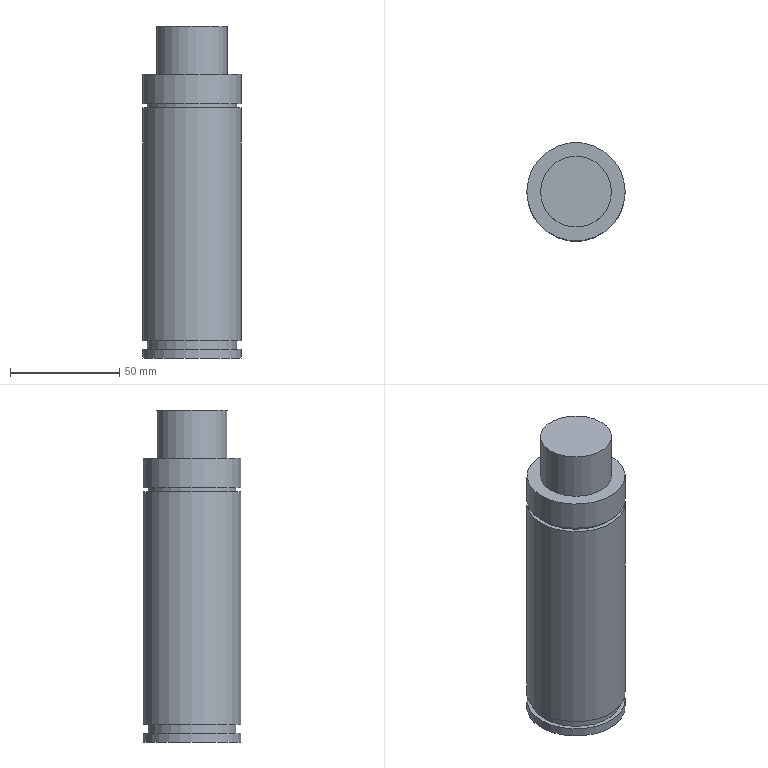Part | NX | features solid 2 | 1 solid | 13 faces | box 45 x 45 x 152 mm | volume 223386 mm3 | plane 7 | cylinder 6 | commonest cylinder face diameters 45 x3 41 x2 32.5 x1
STEP:
#1=CARTESIAN_POINT('',(-897.5,-460.,-46.99));
#2=VERTEX_POINT('',#1);
#3=CARTESIAN_POINT('',(-875.,-460.,-46.99));
#4=DIRECTION('',(0.,0.,1.));
#5=DIRECTION('',(-1.,0.,0.));
#6=AXIS2_PLACEMENT_3D('',#3,#4,#5);
#7=CIRCLE('',#6,22.5);
#8=EDGE_CURVE('',#2,#2,#7,.T.);
#9=ORIENTED_EDGE('',*,*,#8,.T.);
#10=EDGE_LOOP('',(#9));
#11=FACE_BOUND('',#10,.T.);
#12=CARTESIAN_POINT('',(-897.5,-460.,59.51));
#13=VERTEX_POINT('',#12);
#14=CARTESIAN_POINT('',(-875.,-460.,59.51));
#15=DIRECTION('',(0.,0.,1.));
#16=DIRECTION('',(-1.,0.,0.));
#17=AXIS2_PLACEMENT_3D('',#14,#15,#16);
#18=CIRCLE('',#17,22.5);
#19=EDGE_CURVE('',#13,#13,#18,.T.);
#20=ORIENTED_EDGE('',*,*,#19,.F.);
#21=EDGE_LOOP('',(#20));
#22=FACE_BOUND('',#21,.T.);
#23=CARTESIAN_POINT('',(-875.,-460.,-54.99));
#24=DIRECTION('',(0.,0.,1.));
#25=DIRECTION('',(-1.,0.,0.));
#26=AXIS2_PLACEMENT_3D('',#23,#24,#25);
#27=CYLINDRICAL_SURFACE('',#26,22.5);
#28=ADVANCED_FACE('',(#11,#22),#27,.T.);
#29=CARTESIAN_POINT('',(-895.5,-460.,-46.99));
#30=VERTEX_POINT('',#29);
#31=CARTESIAN_POINT('',(-875.,-460.,-46.99));
#32=DIRECTION('',(0.,0.,1.));
#33=DIRECTION('',(-1.,0.,0.));
#34=AXIS2_PLACEMENT_3D('',#31,#32,#33);
#35=CIRCLE('',#34,20.5);
#36=EDGE_CURVE('',#30,#30,#35,.T.);
#37=ORIENTED_EDGE('',*,*,#36,.T.);
#38=EDGE_LOOP('',(#37));
#39=FACE_BOUND('',#38,.T.);
#40=ORIENTED_EDGE('',*,*,#8,.F.);
#41=EDGE_LOOP('',(#40));
#42=FACE_BOUND('',#41,.T.);
#43=CARTESIAN_POINT('',(-875.,-460.,-46.99));
#44=DIRECTION('',(0.,0.,-1.));
#45=DIRECTION('',(1.,0.,0.));
#46=AXIS2_PLACEMENT_3D('',#43,#44,#45);
#47=PLANE('',#46);
#48=ADVANCED_FACE('',(#39,#42),#47,.T.);
#49=CARTESIAN_POINT('',(-895.5,-460.,-50.99));
#50=VERTEX_POINT('',#49);
#51=CARTESIAN_POINT('',(-875.,-460.,-50.99));
#52=DIRECTION('',(0.,0.,1.));
#53=DIRECTION('',(-1.,0.,0.));
#54=AXIS2_PLACEMENT_3D('',#51,#52,#53);
#55=CIRCLE('',#54,20.5);
#56=EDGE_CURVE('',#50,#50,#55,.T.);
#57=ORIENTED_EDGE('',*,*,#56,.F.);
#58=EDGE_LOOP('',(#57));
#59=FACE_BOUND('',#58,.T.);
#60=CARTESIAN_POINT('',(-897.5,-460.,-50.99));
#61=VERTEX_POINT('',#60);
#62=CARTESIAN_POINT('',(-875.,-460.,-50.99));
#63=DIRECTION('',(0.,0.,1.));
#64=DIRECTION('',(-1.,0.,0.));
#65=AXIS2_PLACEMENT_3D('',#62,#63,#64);
#66=CIRCLE('',#65,22.5);
#67=EDGE_CURVE('',#61,#61,#66,.T.);
#68=ORIENTED_EDGE('',*,*,#67,.T.);
#69=EDGE_LOOP('',(#68));
#70=FACE_BOUND('',#69,.T.);
#71=CARTESIAN_POINT('',(-875.,-460.,-50.99));
#72=DIRECTION('',(0.,0.,-1.));
#73=DIRECTION('',(1.,0.,0.));
#74=AXIS2_PLACEMENT_3D('',#71,#72,#73);
#75=PLANE('',#74);
#76=ADVANCED_FACE('',(#59,#70),#75,.F.);
#77=ORIENTED_EDGE('',*,*,#36,.F.);
#78=EDGE_LOOP('',(#77));
#79=FACE_BOUND('',#78,.T.);
#80=ORIENTED_EDGE('',*,*,#56,.T.);
#81=EDGE_LOOP('',(#80));
#82=FACE_BOUND('',#81,.T.);
#83=CARTESIAN_POINT('',(-875.,-460.,-50.99));
#84=DIRECTION('',(0.,0.,1.));
#85=DIRECTION('',(-1.,0.,0.));
#86=AXIS2_PLACEMENT_3D('',#83,#84,#85);
#87=CYLINDRICAL_SURFACE('',#86,20.5);
#88=ADVANCED_FACE('',(#79,#82),#87,.T.);
#89=CARTESIAN_POINT('',(-897.5,-460.,-54.99));
#90=VERTEX_POINT('',#89);
#91=CARTESIAN_POINT('',(-875.,-460.,-54.99));
#92=DIRECTION('',(0.,0.,1.));
#93=DIRECTION('',(-1.,0.,0.));
#94=AXIS2_PLACEMENT_3D('',#91,#92,#93);
#95=CIRCLE('',#94,22.5);
#96=EDGE_CURVE('',#90,#90,#95,.T.);
#97=ORIENTED_EDGE('',*,*,#96,.F.);
#98=EDGE_LOOP('',(#97));
#99=FACE_BOUND('',#98,.T.);
#100=CARTESIAN_POINT('',(-875.,-460.,-54.99));
#101=DIRECTION('',(0.,0.,1.));
#102=DIRECTION('',(-1.,0.,0.));
#103=AXIS2_PLACEMENT_3D('',#100,#101,#102);
#104=PLANE('',#103);
#105=ADVANCED_FACE('',(#99),#104,.F.);
#106=ORIENTED_EDGE('',*,*,#96,.T.);
#107=EDGE_LOOP('',(#106));
#108=FACE_BOUND('',#107,.T.);
#109=ORIENTED_EDGE('',*,*,#67,.F.);
#110=EDGE_LOOP('',(#109));
#111=FACE_BOUND('',#110,.T.);
#112=CARTESIAN_POINT('',(-875.,-460.,-54.99));
#113=DIRECTION('',(0.,0.,1.));
#114=DIRECTION('',(-1.,0.,0.));
#115=AXIS2_PLACEMENT_3D('',#112,#113,#114);
#116=CYLINDRICAL_SURFACE('',#115,22.5);
#117=ADVANCED_FACE('',(#108,#111),#116,.T.);
#118=CARTESIAN_POINT('',(-854.5,-460.,59.51));
#119=VERTEX_POINT('',#118);
#120=CARTESIAN_POINT('',(-875.,-460.,59.51));
#121=DIRECTION('',(0.,0.,-1.));
#122=DIRECTION('',(1.,0.,0.));
#123=AXIS2_PLACEMENT_3D('',#120,#121,#122);
#124=CIRCLE('',#123,20.5);
#125=EDGE_CURVE('',#119,#119,#124,.F.);
#126=ORIENTED_EDGE('',*,*,#125,.F.);
#127=EDGE_LOOP('',(#126));
#128=FACE_BOUND('',#127,.T.);
#129=ORIENTED_EDGE('',*,*,#19,.T.);
#130=EDGE_LOOP('',(#129));
#131=FACE_BOUND('',#130,.T.);
#132=CARTESIAN_POINT('',(-875.,-460.,59.51));
#133=DIRECTION('',(0.,0.,-1.));
#134=DIRECTION('',(1.,0.,0.));
#135=AXIS2_PLACEMENT_3D('',#132,#133,#134);
#136=PLANE('',#135);
#137=ADVANCED_FACE('',(#128,#131),#136,.F.);
#138=CARTESIAN_POINT('',(-854.5,-460.,61.51));
#139=VERTEX_POINT('',#138);
#140=CARTESIAN_POINT('',(-875.,-460.,61.51));
#141=DIRECTION('',(0.,0.,-1.));
#142=DIRECTION('',(1.,0.,0.));
#143=AXIS2_PLACEMENT_3D('',#140,#141,#142);
#144=CIRCLE('',#143,20.5);
#145=EDGE_CURVE('',#139,#139,#144,.F.);
#146=ORIENTED_EDGE('',*,*,#145,.T.);
#147=EDGE_LOOP('',(#146));
#148=FACE_BOUND('',#147,.T.);
#149=CARTESIAN_POINT('',(-897.5,-460.,61.51));
#150=VERTEX_POINT('',#149);
#151=CARTESIAN_POINT('',(-875.,-460.,61.51));
#152=DIRECTION('',(0.,0.,1.));
#153=DIRECTION('',(-1.,0.,0.));
#154=AXIS2_PLACEMENT_3D('',#151,#152,#153);
#155=CIRCLE('',#154,22.5);
#156=EDGE_CURVE('',#150,#150,#155,.T.);
#157=ORIENTED_EDGE('',*,*,#156,.F.);
#158=EDGE_LOOP('',(#157));
#159=FACE_BOUND('',#158,.T.);
#160=CARTESIAN_POINT('',(-875.,-460.,61.51));
#161=DIRECTION('',(0.,0.,-1.));
#162=DIRECTION('',(1.,0.,0.));
#163=AXIS2_PLACEMENT_3D('',#160,#161,#162);
#164=PLANE('',#163);
#165=ADVANCED_FACE('',(#148,#159),#164,.T.);
#166=ORIENTED_EDGE('',*,*,#125,.T.);
#167=EDGE_LOOP('',(#166));
#168=FACE_BOUND('',#167,.T.);
#169=ORIENTED_EDGE('',*,*,#145,.F.);
#170=EDGE_LOOP('',(#169));
#171=FACE_BOUND('',#170,.T.);
#172=CARTESIAN_POINT('',(-875.,-460.,61.51));
#173=DIRECTION('',(0.,0.,-1.));
#174=DIRECTION('',(1.,0.,0.));
#175=AXIS2_PLACEMENT_3D('',#172,#173,#174);
#176=CYLINDRICAL_SURFACE('',#175,20.5);
#177=ADVANCED_FACE('',(#168,#171),#176,.T.);
#178=CARTESIAN_POINT('',(-891.25,-460.,75.01));
#179=VERTEX_POINT('',#178);
#180=CARTESIAN_POINT('',(-875.,-460.,75.01));
#181=DIRECTION('',(0.,0.,1.));
#182=DIRECTION('',(-1.,0.,0.));
#183=AXIS2_PLACEMENT_3D('',#180,#181,#182);
#184=CIRCLE('',#183,16.25);
#185=EDGE_CURVE('',#179,#179,#184,.T.);
#186=ORIENTED_EDGE('',*,*,#185,.F.);
#187=EDGE_LOOP('',(#186));
#188=FACE_BOUND('',#187,.T.);
#189=CARTESIAN_POINT('',(-897.5,-460.,75.01));
#190=VERTEX_POINT('',#189);
#191=CARTESIAN_POINT('',(-875.,-460.,75.01));
#192=DIRECTION('',(0.,0.,1.));
#193=DIRECTION('',(-1.,0.,0.));
#194=AXIS2_PLACEMENT_3D('',#191,#192,#193);
#195=CIRCLE('',#194,22.5);
#196=EDGE_CURVE('',#190,#190,#195,.T.);
#197=ORIENTED_EDGE('',*,*,#196,.T.);
#198=EDGE_LOOP('',(#197));
#199=FACE_BOUND('',#198,.T.);
#200=CARTESIAN_POINT('',(-875.,-460.,75.01));
#201=DIRECTION('',(0.,0.,1.));
#202=DIRECTION('',(-1.,0.,0.));
#203=AXIS2_PLACEMENT_3D('',#200,#201,#202);
#204=PLANE('',#203);
#205=ADVANCED_FACE('',(#188,#199),#204,.T.);
#206=ORIENTED_EDGE('',*,*,#196,.F.);
#207=EDGE_LOOP('',(#206));
#208=FACE_BOUND('',#207,.T.);
#209=ORIENTED_EDGE('',*,*,#156,.T.);
#210=EDGE_LOOP('',(#209));
#211=FACE_BOUND('',#210,.T.);
#212=CARTESIAN_POINT('',(-875.,-460.,-54.99));
#213=DIRECTION('',(0.,0.,1.));
#214=DIRECTION('',(-1.,0.,0.));
#215=AXIS2_PLACEMENT_3D('',#212,#213,#214);
#216=CYLINDRICAL_SURFACE('',#215,22.5);
#217=ADVANCED_FACE('',(#208,#211),#216,.T.);
#218=ORIENTED_EDGE('',*,*,#185,.T.);
#219=EDGE_LOOP('',(#218));
#220=FACE_BOUND('',#219,.T.);
#221=CARTESIAN_POINT('',(-858.75,-460.,97.01));
#222=VERTEX_POINT('',#221);
#223=CARTESIAN_POINT('',(-875.,-460.,97.01));
#224=DIRECTION('',(0.,0.,1.));
#225=DIRECTION('',(1.,0.,0.));
#226=AXIS2_PLACEMENT_3D('',#223,#224,#225);
#227=CIRCLE('',#226,16.25);
#228=EDGE_CURVE('',#222,#222,#227,.T.);
#229=ORIENTED_EDGE('',*,*,#228,.F.);
#230=EDGE_LOOP('',(#229));
#231=FACE_BOUND('',#230,.T.);
#232=CARTESIAN_POINT('',(-875.,-460.,55.01));
#233=DIRECTION('',(0.,0.,1.));
#234=DIRECTION('',(-1.,0.,0.));
#235=AXIS2_PLACEMENT_3D('',#232,#233,#234);
#236=CYLINDRICAL_SURFACE('',#235,16.25);
#237=ADVANCED_FACE('',(#220,#231),#236,.T.);
#238=ORIENTED_EDGE('',*,*,#228,.T.);
#239=EDGE_LOOP('',(#238));
#240=FACE_BOUND('',#239,.T.);
#241=CARTESIAN_POINT('',(-875.,-460.,97.01));
#242=DIRECTION('',(0.,0.,1.));
#243=DIRECTION('',(-1.,0.,0.));
#244=AXIS2_PLACEMENT_3D('',#241,#242,#243);
#245=PLANE('',#244);
#246=ADVANCED_FACE('',(#240),#245,.T.);
#247=CLOSED_SHELL('',(#28,#48,#76,#88,#105,#117,#137,#165,#177,#205,#217,#237,#246));
#248=MANIFOLD_SOLID_BREP('',#247);
#249=(LENGTH_UNIT()NAMED_UNIT(*)SI_UNIT(.MILLI.,.METRE.));
#250=UNCERTAINTY_MEASURE_WITH_UNIT(LENGTH_MEASURE(0.00001),#249,'','');
#251=(NAMED_UNIT(*)PLANE_ANGLE_UNIT()SI_UNIT($,.RADIAN.));
#252=(NAMED_UNIT(*)SI_UNIT($,.STERADIAN.)SOLID_ANGLE_UNIT());
#253=(GEOMETRIC_REPRESENTATION_CONTEXT(3)GLOBAL_UNCERTAINTY_ASSIGNED_CONTEXT((#250))GLOBAL_UNIT_ASSIGNED_CONTEXT((#249,#251,#252))REPRESENTATION_CONTEXT('',''));
#254=ADVANCED_BREP_SHAPE_REPRESENTATION('',(#248),#253);